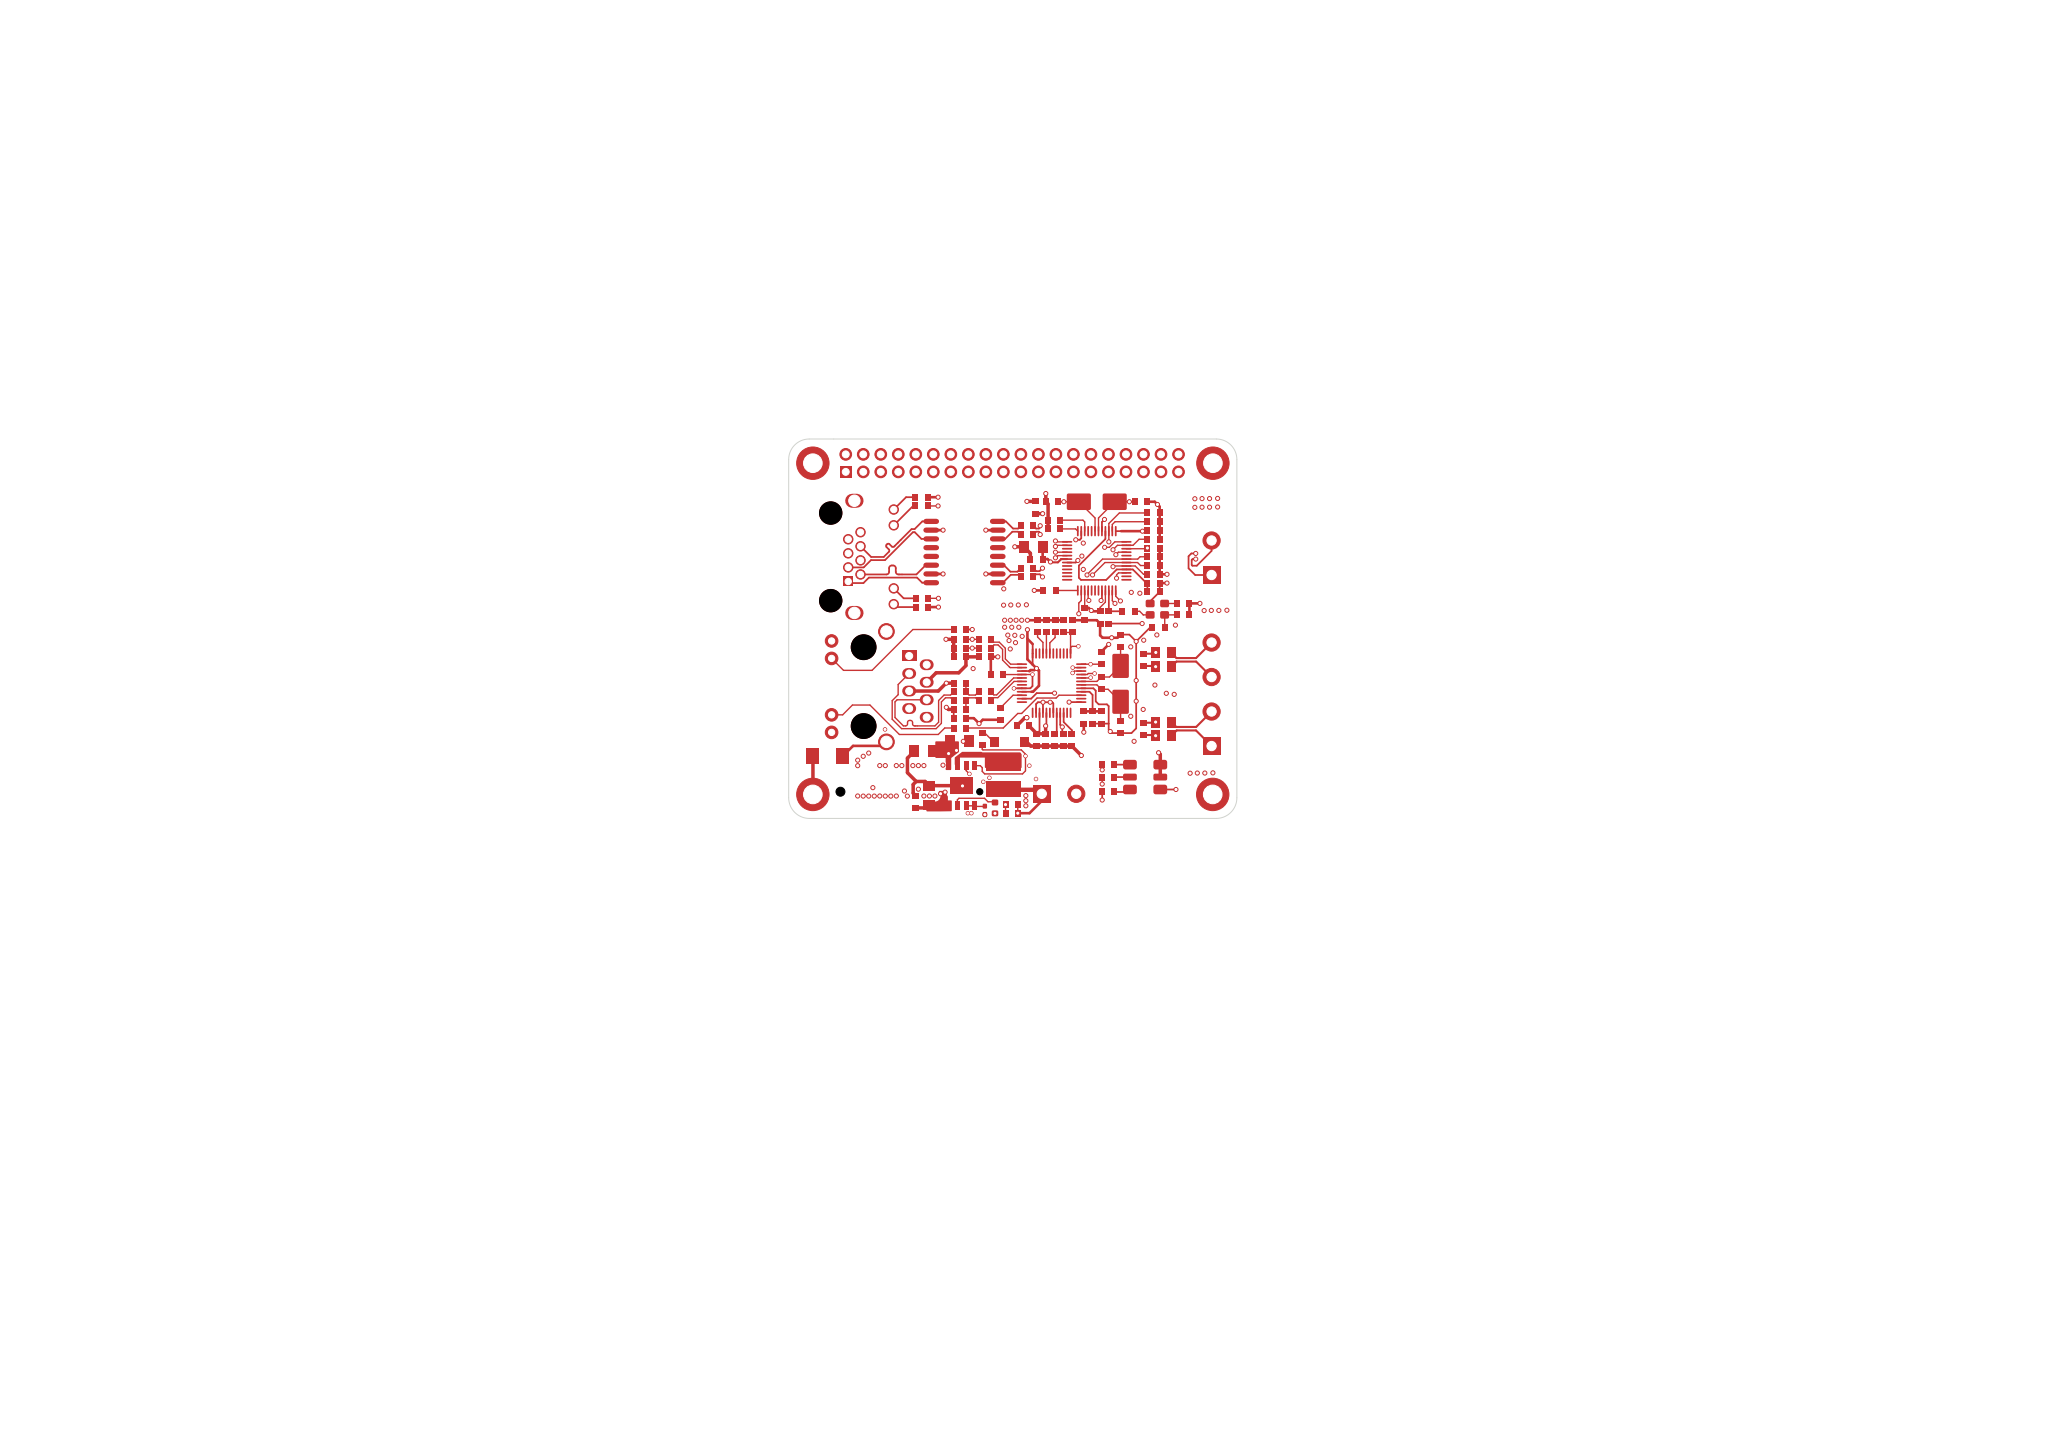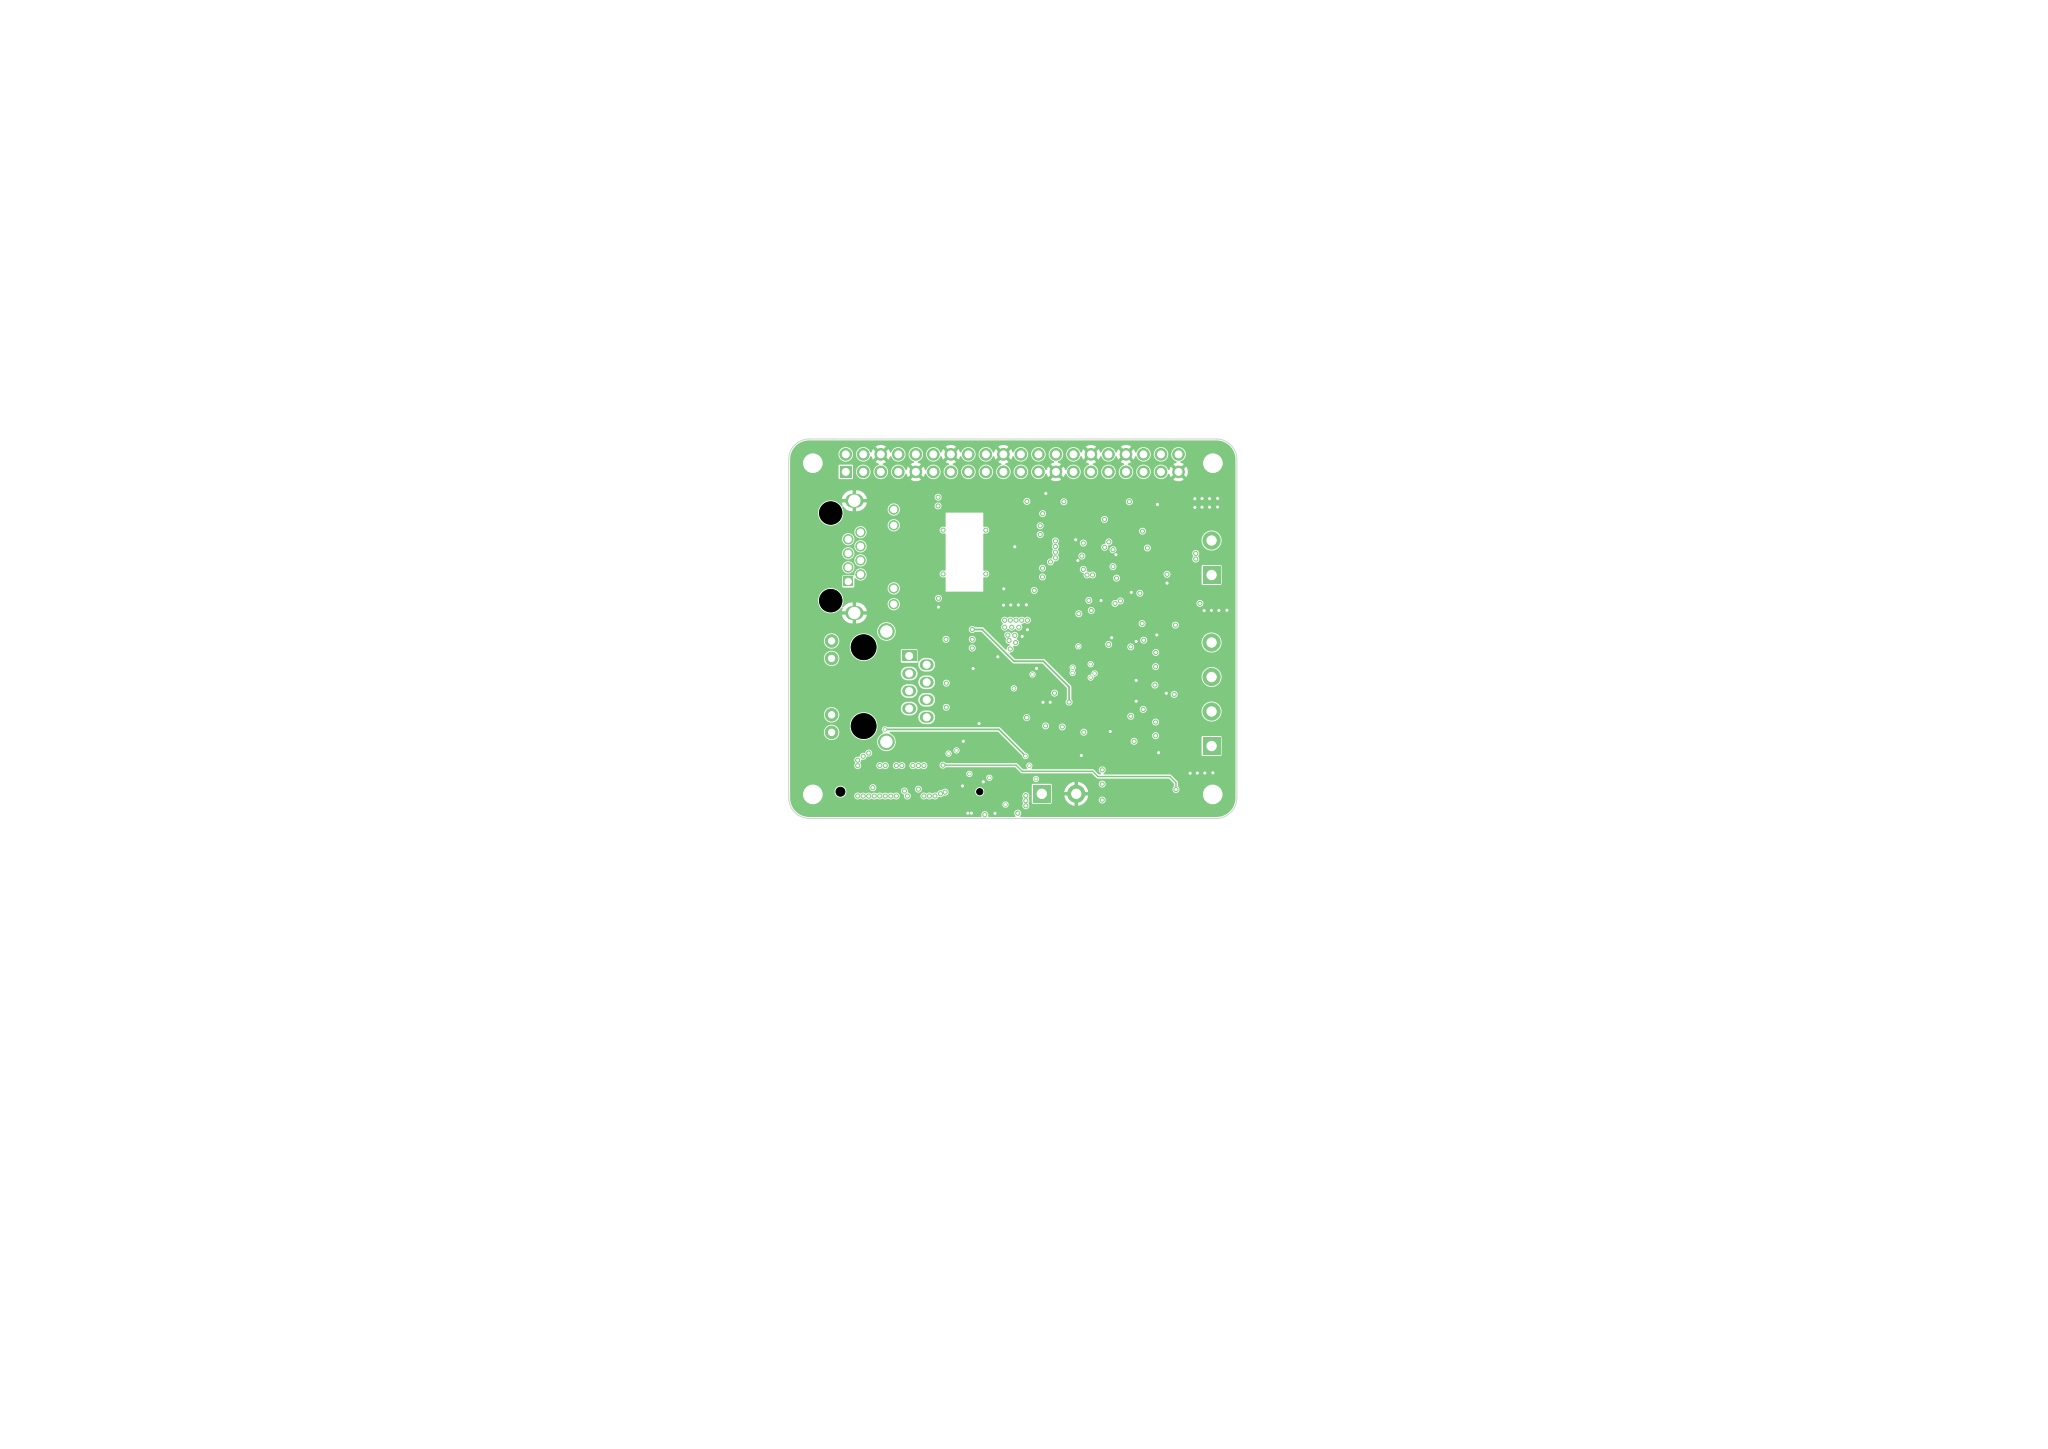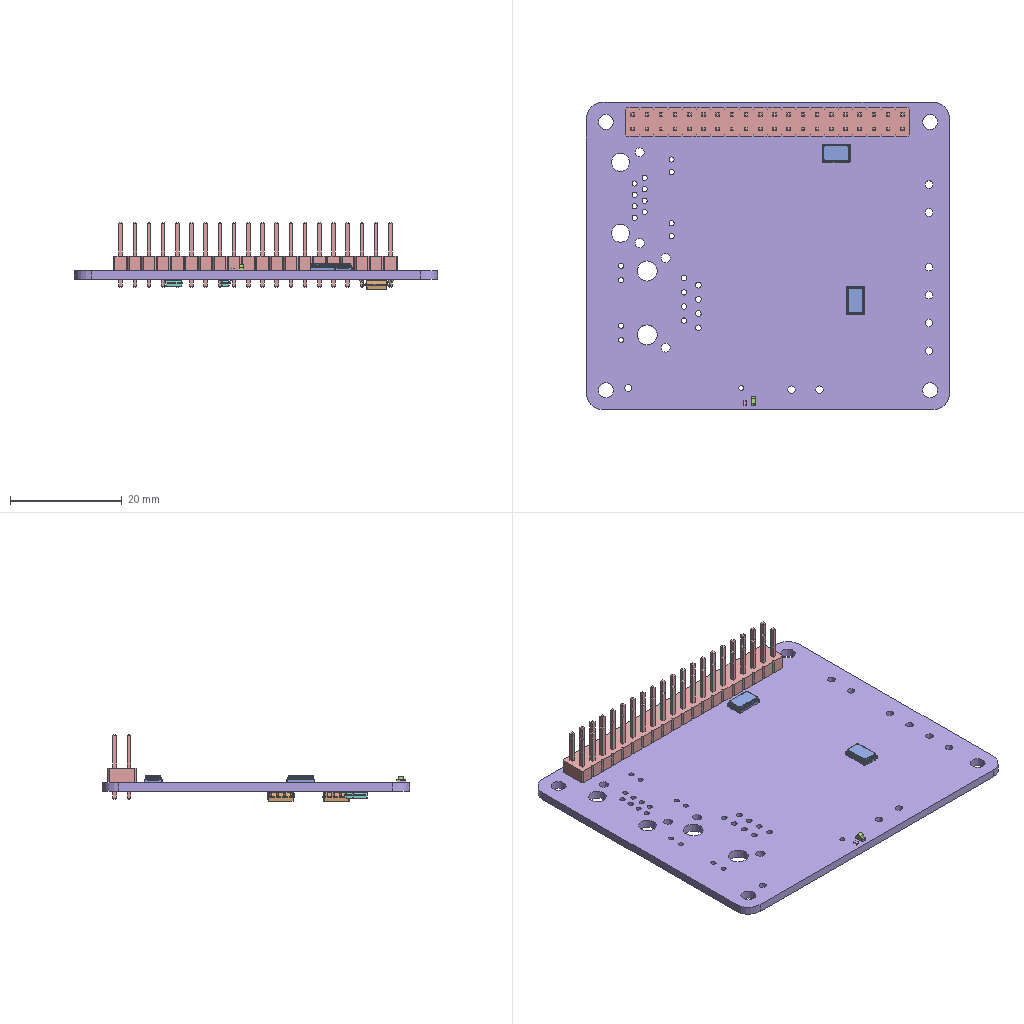Circuit board layout | KiCad | box 65 x 55 x 12 mm
Layer stack:
layer,type,thickness_mm,material,epsilon_r
F.SilkS,Top Silk Screen,,,
F.Paste,Top Solder Paste,,,
F.Mask,Top Solder Mask,0.01,,
F.Cu,copper,0.035,,
dielectric 1,prepreg,0.1,FR4,4.5
In1.Cu,copper,0.035,,
dielectric 2,core,0.535,FR4,4.5
In2.Cu,copper,0.035,,
dielectric 3,prepreg,0.1,FR4,4.5
In3.Cu,copper,0.035,,
dielectric 4,core,0.535,FR4,4.5
In4.Cu,copper,0.035,,
dielectric 5,prepreg,0.1,FR4,4.5
B.Cu,copper,0.035,,
B.Mask,Bottom Solder Mask,0.01,,
B.Paste,Bottom Solder Paste,,,
B.SilkS,Bottom Silk Screen,,,
Part placement:
Ref,Val,Package,PosX,PosY,Rot,Side
C1,0.1u,C0603,164.059,-84.43,0,bottom
C2,0.1u,C0603,170.028,-102.006,0,bottom
C3,0.1u,C0603,164.059,-76.556,180,bottom
C4,0.1u,C0603,163.982,-105.562,90,bottom
C5,0.1u,C0603,170.053,-92.024,0,bottom
C6,0.1u,C0603,163.982,-95.555,90,bottom
C16,22u,C1206,138.049,-105.258,0,bottom
C17,22u,C1206,152.298,-109.474,0,bottom
C22,0.1u,C0603,162.204,-75.286,180,bottom
C33,0.1u,C0603,144.678,-83.185,180,bottom
C34,0.1u,C0603,144.678,-76.835,180,bottom
C35,0.1u,C0603,135.001,-76.835,0,bottom
C36,0.1u,C0603,135.026,-83.185,0,bottom
C37,22u,C1206,152.298,-111.76,0,bottom
C38,0.1u,C0603,138.709,-109.652,90,bottom
C39,1nF/2000V,C1808,132.131,-73.939,90,bottom
C40,0.1u,C0603,145.745,-114.148,0,bottom
C42,22u,C1206,145.796,-96.901,180,bottom
C43,22u,C1206,145.796,-99.212,180,bottom
C44,0.1u,C0603,145.339,-101.092,0,bottom
C45,10p,C0603,143.027,-103.988,90,bottom
C172,0.1u,C0603,149.911,-100.152,-90,bottom
C173,0.1u,C0603,148.234,-97.485,-90,bottom
CN1,X0802FVS-40AS-LPV01,CONN-SMD_40P-P0.80-Mu,132.178,-114.747,0,bottom
L5,6.8uH/1.5A,PL0505,147.828,-107.074,0,bottom
Q1,AO3401A,SOT-23,141.402,-109.601,0,bottom
Q2,2N7002,SOT-23,132.156,-107.874,-90,bottom
R1,1k,R0603,167.615,-77.318,90,bottom
R2,1k,R0603,170.028,-109.093,0,bottom
R5,2.2,R0805,170.663,-79.604,0,bottom
R7,1k,R0603,170.028,-99.162,0,bottom
R23,1k,R0603,167.615,-83.922,90,bottom
R24,1M,R0603,159.055,-72.72,180,bottom
R25,3.3K,R0603,135.56,-109.068,0,bottom
R26,2.2,R0805,170.663,-81.636,0,bottom
R27,120,R0603,167.615,-80.62,90,bottom
R38,1k,R0603,130.327,-105.156,0,bottom
R39,10K,R0603,135.585,-107.29,0,bottom
R40,10K,R0603,147.599,-111.379,-90,bottom
R41,100K 1%,R0603,144.297,-103.988,90,bottom
R42,22.1K,R0603,144.297,-106.934,90,bottom
R52,75,R0805,132.969,-78.537,0,bottom
R53,75,R0805,132.994,-81.483,0,bottom
U1,SY8031AAC,SOT23-5-I38-100,145.263,-110.998,180,bottom
U2,TJA1051T-3,SOIC-8_3.9x4.9mm_P1.27mm,168.453,-95.564,0,bottom
U3,TJA1051T-3,SOIC-8_3.9x4.9mm_P1.27mm,168.453,-105.546,0,bottom
U7,SP3072,SO8_D_R-PDSO-G8,161.519,-80.62,90,bottom
C7,0.1u,C0603,168.021,-90.881,0,top
C12,22u,C1206,134.772,-116.662,90,top
C13,0.1u,C0603,132.791,-116.205,-90,top
C14,22u,C1206,137.795,-107.442,0,top
C15,22u,C1206,135.357,-108.915,180,top
C18,15p,C0603,165.456,-72.72,0,top
C20,15p,C0603,152.552,-72.72,180,top
C21,0.1u,C0603,150.317,-81.026,0,top
C23,4.7u,C1206,148.488,-79.248,0,top
C24,0.1u,C0603,157.302,-89.002,90,top
C25,0.1u,C0603,159.537,-89.484,90,top
C26,0.1u,C0603,167.284,-76.886,180,top
C28,4.7u,C0603,167.284,-84.506,180,top
C30,0.1u,C0603,167.284,-85.776,180,top
C32,0.1u,C0603,152.883,-76.657,0,top
C161,18p,C0603,162.509,-105.359,-90,top
C162,18p,C0603,162.509,-92.862,90,top
C163,6.8n,C0603,139.192,-101.549,0,top
C164,6.8n,C0603,139.192,-100.279,0,top
C165,10n,C0603,139.192,-104.089,180,top
C166,1n,C0603,155.55,-90.78,-90,top
C167,0.1u,C0603,158.445,-103.988,90,top
C168,4.7u,C0603,159.715,-103.988,90,top
C169,22n,C0603,142.799,-95.199,0,top
C170,0.1u,C0603,144.577,-97.739,0,top
C171,0.1u,C0603,151.638,-107.239,90,top
C174,4.7u,C0603,150.368,-107.239,90,top
C175,1nF/2000V,C1808,120.066,-109.576,180,top
C176,0.1u,C0603,154.178,-107.239,90,top
C178,4.7u,C0603,152.908,-107.239,-90,top
C179,0.1u,C0603,155.448,-107.239,90,top
CN2,KF301-4P,HEAD4L-0.8,175.704,-108.124,90,top
CN3,KF301-2P,HEAD2L-0.8,175.704,-83.337,90,top
CN4,KF301-2P,HEAD2L-0.8,151.079,-115.049,0,top
D1,Inolux_IN-P55TATRGB,LED_Inolux_IN-P55TATRGB_PLCC6_5.0x5.5mm_P1.8mm,166.065,-112.624,180,top
D3,LED,LED_0603_1608Metric,144.297,-117.094,90,top
J1,Conn_02x20_Odd_Even,PinHeader_2x20_P2.54mm_Vertical,122.65,-68.39,90,top
J2,RJ45,RJ45_1X1L_20U,122.631,-80.594,-90,top
L1,L0603,L0603,171.602,-89.103,180,top
L2,L0603,L0603,150.165,-73.558,90,top
L3,L0603,L0603,157.175,-103.988,-90,top
L4,1uH/3.8A,PL0505,145.544,-110.549,0,top
L8,L0603,L0603,148.336,-105.207,180,top
R3,120,R0603,165.786,-105.639,90,top
R4,2.2,R0805,168.732,-106.629,0,top
R6,2.2,R0805,168.732,-104.648,0,top
R8,1.5K,R0603,167.284,-81.966,0,top
R9,10K,R0603,152.197,-85.573,180,top
R10,1.5K,R0603,160.731,-110.82,180,top
R11,1.5K,R0603,160.731,-112.624,180,top
R12,120,R0603,165.786,-95.631,90,top
R13,2.2,R0805,168.732,-96.622,0,top
R14,2.2,R0805,168.732,-94.64,0,top
R15,33,R0603,160.807,-89.484,90,top
R16,33,R0603,163.652,-88.595,180,top
R17,10K,R0603,171.602,-87.452,180,top
R18,1K,R_0402_1005Metric_Pad0.72x0.64mm_HandSolder,142.824,-117.438,90,top
R19,10K,R0603,160.731,-114.783,180,top
R20,1,R0603,146.71,-117.856,0,top
R21,1,R0603,146.71,-116.586,0,top
R22,10K,R0603,142.443,-107.137,-90,top
R28,10K,R0603,167.284,-83.236,0,top
R29,2.2,R0603,148.946,-83.617,180,top
R30,2.2,R0603,148.946,-82.347,180,top
R31,1.5K,R0603,167.284,-80.696,0,top
R32,2.2,R0603,148.946,-77.47,180,top
R33,2.2,R0603,148.946,-76.2,180,top
R34,510,R0603,133.655,-73.33,180,top
R35,10K,R0603,167.284,-79.426,0,top
R36,1K,R0603,167.284,-78.156,0,top
R37,510,R0603,133.68,-86.716,180,top
R46,2.49K 1%,R0603,152.883,-75.387,0,top
R48,1K,R0603,167.284,-75.616,180,top
R49,1K,R0603,167.284,-74.346,180,top
R50,0,R0603,133.68,-87.986,0,top
R51,0,R0603,133.655,-72.06,0,top
R179,10,R0603,139.192,-95.199,0,top
R180,1M,R0603,159.715,-99.009,90,top
R181,49.9,R0603,139.192,-93.929,0,top
R182,49.9,R0603,139.192,-92.659,0,top
R183,3.3,R0603,142.799,-93.929,0,top
R185,3.3,R0603,142.799,-92.659,0,top
R186,3.3,R0603,142.799,-101.549,0,top
R187,3.3,R0603,142.799,-100.279,0,top
R188,10K,R0603,154.28,-90.78,90,top
R190,49.9,R0603,139.192,-102.819,180,top
R191,49.9,R0603,139.192,-99.009,180,top
R192,10K,R0603,159.69,-95.377,90,top
R193,330,R0603,139.192,-91.237,0,top
R194,10K,R0603,150.47,-90.78,90,top
R195,10K,R0603,151.74,-90.78,90,top
R196,330,R0603,139.192,-105.512,0,top
R197,10K,R0603,153.01,-90.78,90,top
R198,12.4K 1%,R0603,145.136,-103.429,-90,top
SW1,TS-1088R-02026,SW-SMD_L3.9-W3.0-P4.45,146.355,-107.594,0,top
T2,TS6121C,TS6121C,139.871,-80.01,90,top
U4,RTL8201EL-VC-GR,P48LQFP,159.055,-81.28,-90,top
U5,IP5306,ESOP-8_L4.9-W3.9-P1.27-LS6.0-BL-EP,139.471,-113.881,0,top
U20,W5500,P48LQFP,152.502,-99.009,-90,top
U21,HR911105A,HR911105A,120.953,-99.111,180,top
Y1,ASE-50MHz,Oscillator_SMD_Abracon_ASE-4Pin_3.2x2.5mm,167.843,-88.29,180,top
Y3,25Mhz,Crystal_SMD_5032-2Pin_5.0x3.2mm_HandSoldering,159.055,-72.72,0,top
Y4,25Mhz,Crystal_SMD_5032-2Pin_5.0x3.2mm_HandSoldering,162.509,-99.111,-90,top
Pad and via stacks:
via_type,start_layer,end_layer,diameter_mm,drill_mm,count
through,F.Cu,B.Cu,0.5,0.3,21
through,F.Cu,B.Cu,0.6,0.3,173
Design rules, without the lines most boards share:
# KiCad design rules of  (from the KiCad project file, unit mm)
max_error = 0.005
min_clearance = 0.0
min_connection = 0.0
min_copper_edge_clearance = 0.2032
min_groove_width = 0.0
min_hole_clearance = 0.2032
min_hole_to_hole = 0.25
min_microvia_diameter = 0.2
min_microvia_drill = 0.1
min_resolved_spokes = 2
min_silk_clearance = 0.0
min_text_height = 0.8
min_text_thickness = 0.08
min_through_hole_diameter = 0.3
min_track_width = 0.0
min_via_annular_width = 0.1
min_via_diameter = 0.5
solder_mask_to_copper_clearance = 0.0
use_height_for_length_calcs = True
defaults = {"apply_defaults_to_fp_fields": false, "apply_defaults_to_fp_shapes": false, "apply_defaults_to_fp_text": false, "board_outline_line_width": 0.05, "copper_line_width": 0.2, "copper_text_italic": false, "copper_text_size_h": 1.5, "copper_text_size_v": 1.5, "copper_text_thickness": 0.3, "copper_text_upright": false, "courtyard_line_width": 0.05, "dimension_precision": 4, "dimension_units": 3, "dimensions": {"arrow_length": 1270000, "extension_offset": 500000, "keep_text_aligned": true, "suppress_zeroes": true, "text_position": 0, "units_format": 0}, "fab_line_width": 0.1, "fab_text_italic": false, "fab_text_size_h": 1.0, "fab_text_size_v": 1.0, "fab_text_thickness": 0.15, "fab_text_upright": false, "other_line_width": 0.1, "other_text_italic": false, "other_text_size_h": 1.0, "other_text_size_v": 1.0, "other_text_thickness": 0.15, "other_text_upright": false, "pads": {"drill": 2.7, "height": 3.1, "width": 3.1}, "silk_line_width": 0.1, "silk_text_italic": false, "silk_text_size_h": 1.0, "silk_text_size_v": 1.0, "silk_text_thickness": 0.1, "silk_text_upright": false, "zones": {"min_clearance": 0.0}}
track_widths = [0.0]
via_dimensions = [{"diameter": 0.0, "drill": 0.0}]
diff_pair_dimensions = [{"gap": 0.0, "via_gap": 0.0, "width": 0.0}]
# copper zones (pour): pad connection, clearance mm, minimum width mm, count
Classes set for this board:
# KiCad net classes of  (from the KiCad project file, unit mm)
{"bus_width": 12, "clearance": 0.2, "diff_pair_gap": 0.25, "diff_pair_via_gap": 0.25, "diff_pair_width": 0.2, "line_style": 0, "microvia_diameter": 0.3, "microvia_drill": 0.1, "name": "Default", "pcb_color": "rgba(0, 0, 0, 0.000)", "priority": 2147483647, "schematic_color": "rgba(0, 0, 0, 0.000)", "track_width": 0.2, "via_diameter": 0.6, "via_drill": 0.3, "wire_width": 6}